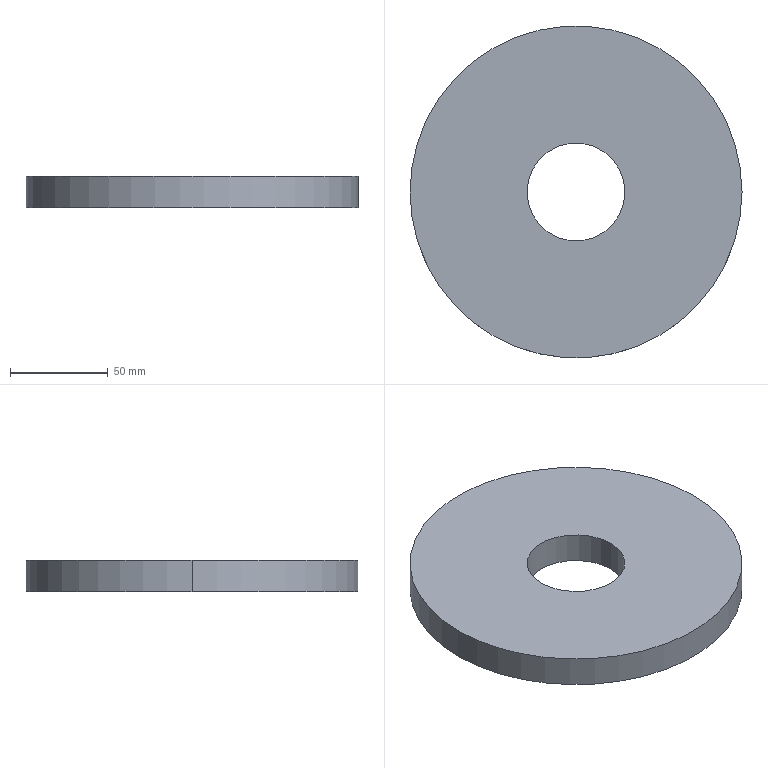Part | SolidWorks | features Extrusion 1 | 1 solid | 6 faces | box 169.5 x 169.5 x 16 mm | volume 329619 mm3 | cylinder 4 | plane 2 | commonest cylinder face diameters 50 x2 169.5 x2
STEP:
#1=CARTESIAN_POINT('',(-25.,0.,16.));
#2=VERTEX_POINT('',#1);
#3=CARTESIAN_POINT('',(25.,0.,16.));
#4=VERTEX_POINT('',#3);
#5=CARTESIAN_POINT('',(0.,0.,16.));
#6=DIRECTION('',(0.,0.,1.));
#7=DIRECTION('',(1.,0.,0.));
#8=AXIS2_PLACEMENT_3D('',#5,#6,#7);
#9=CIRCLE('',#8,25.);
#10=EDGE_CURVE('',#2,#4,#9,.T.);
#11=ORIENTED_EDGE('',*,*,#10,.T.);
#12=CARTESIAN_POINT('',(25.,0.,0.));
#13=VERTEX_POINT('',#12);
#14=CARTESIAN_POINT('',(25.,0.,16.));
#15=DIRECTION('',(0.,0.,-1.));
#16=VECTOR('',#15,1000.);
#17=LINE('',#14,#16);
#18=EDGE_CURVE('',#4,#13,#17,.T.);
#19=ORIENTED_EDGE('',*,*,#18,.T.);
#20=CARTESIAN_POINT('',(-25.,0.,0.));
#21=VERTEX_POINT('',#20);
#22=CARTESIAN_POINT('',(0.,0.,0.));
#23=DIRECTION('',(0.,0.,1.));
#24=DIRECTION('',(1.,0.,0.));
#25=AXIS2_PLACEMENT_3D('',#22,#23,#24);
#26=CIRCLE('',#25,25.);
#27=EDGE_CURVE('',#21,#13,#26,.T.);
#28=ORIENTED_EDGE('',*,*,#27,.F.);
#29=CARTESIAN_POINT('',(-25.,0.,16.));
#30=DIRECTION('',(0.,0.,-1.));
#31=VECTOR('',#30,1000.);
#32=LINE('',#29,#31);
#33=EDGE_CURVE('',#2,#21,#32,.T.);
#34=ORIENTED_EDGE('',*,*,#33,.F.);
#35=EDGE_LOOP('',(#11,#19,#28,#34));
#36=FACE_OUTER_BOUND('',#35,.T.);
#37=CARTESIAN_POINT('',(0.,0.,16.));
#38=DIRECTION('',(0.,0.,-1.));
#39=DIRECTION('',(-1.,0.,0.));
#40=AXIS2_PLACEMENT_3D('',#37,#38,#39);
#41=CYLINDRICAL_SURFACE('',#40,25.);
#42=ADVANCED_FACE('',(#36),#41,.F.);
#43=CARTESIAN_POINT('',(84.75,0.,16.));
#44=VERTEX_POINT('',#43);
#45=CARTESIAN_POINT('',(-84.75,0.,16.));
#46=VERTEX_POINT('',#45);
#47=CARTESIAN_POINT('',(0.,0.,16.));
#48=DIRECTION('',(0.,0.,1.));
#49=DIRECTION('',(1.,0.,0.));
#50=AXIS2_PLACEMENT_3D('',#47,#48,#49);
#51=CIRCLE('',#50,84.75);
#52=EDGE_CURVE('',#44,#46,#51,.T.);
#53=ORIENTED_EDGE('',*,*,#52,.F.);
#54=CARTESIAN_POINT('',(84.75,0.,0.));
#55=VERTEX_POINT('',#54);
#56=CARTESIAN_POINT('',(84.75,0.,16.));
#57=DIRECTION('',(0.,0.,-1.));
#58=VECTOR('',#57,1000.);
#59=LINE('',#56,#58);
#60=EDGE_CURVE('',#44,#55,#59,.T.);
#61=ORIENTED_EDGE('',*,*,#60,.T.);
#62=CARTESIAN_POINT('',(-84.75,0.,0.));
#63=VERTEX_POINT('',#62);
#64=CARTESIAN_POINT('',(0.,0.,0.));
#65=DIRECTION('',(0.,0.,1.));
#66=DIRECTION('',(1.,0.,0.));
#67=AXIS2_PLACEMENT_3D('',#64,#65,#66);
#68=CIRCLE('',#67,84.75);
#69=EDGE_CURVE('',#55,#63,#68,.T.);
#70=ORIENTED_EDGE('',*,*,#69,.T.);
#71=CARTESIAN_POINT('',(-84.75,0.,16.));
#72=DIRECTION('',(0.,0.,-1.));
#73=VECTOR('',#72,1000.);
#74=LINE('',#71,#73);
#75=EDGE_CURVE('',#46,#63,#74,.T.);
#76=ORIENTED_EDGE('',*,*,#75,.F.);
#77=EDGE_LOOP('',(#53,#61,#70,#76));
#78=FACE_OUTER_BOUND('',#77,.T.);
#79=CARTESIAN_POINT('',(0.,0.,16.));
#80=DIRECTION('',(0.,0.,-1.));
#81=DIRECTION('',(-1.,0.,0.));
#82=AXIS2_PLACEMENT_3D('',#79,#80,#81);
#83=CYLINDRICAL_SURFACE('',#82,84.75);
#84=ADVANCED_FACE('',(#78),#83,.T.);
#85=CARTESIAN_POINT('',(0.,0.,16.));
#86=DIRECTION('',(0.,0.,1.));
#87=DIRECTION('',(1.,0.,0.));
#88=AXIS2_PLACEMENT_3D('',#85,#86,#87);
#89=CIRCLE('',#88,84.75);
#90=EDGE_CURVE('',#46,#44,#89,.T.);
#91=ORIENTED_EDGE('',*,*,#90,.T.);
#92=ORIENTED_EDGE('',*,*,#52,.T.);
#93=EDGE_LOOP('',(#91,#92));
#94=FACE_OUTER_BOUND('',#93,.T.);
#95=ORIENTED_EDGE('',*,*,#10,.F.);
#96=CARTESIAN_POINT('',(0.,0.,16.));
#97=DIRECTION('',(0.,0.,1.));
#98=DIRECTION('',(1.,0.,0.));
#99=AXIS2_PLACEMENT_3D('',#96,#97,#98);
#100=CIRCLE('',#99,25.);
#101=EDGE_CURVE('',#4,#2,#100,.T.);
#102=ORIENTED_EDGE('',*,*,#101,.F.);
#103=EDGE_LOOP('',(#95,#102));
#104=FACE_BOUND('',#103,.T.);
#105=CARTESIAN_POINT('',(0.,0.,16.));
#106=DIRECTION('',(0.,0.,1.));
#107=DIRECTION('',(1.,0.,0.));
#108=AXIS2_PLACEMENT_3D('',#105,#106,#107);
#109=PLANE('',#108);
#110=ADVANCED_FACE('',(#94,#104),#109,.T.);
#111=CARTESIAN_POINT('',(0.,0.,0.));
#112=DIRECTION('',(0.,0.,1.));
#113=DIRECTION('',(1.,0.,0.));
#114=AXIS2_PLACEMENT_3D('',#111,#112,#113);
#115=CIRCLE('',#114,84.75);
#116=EDGE_CURVE('',#63,#55,#115,.T.);
#117=ORIENTED_EDGE('',*,*,#116,.F.);
#118=ORIENTED_EDGE('',*,*,#69,.F.);
#119=EDGE_LOOP('',(#117,#118));
#120=FACE_OUTER_BOUND('',#119,.T.);
#121=ORIENTED_EDGE('',*,*,#27,.T.);
#122=CARTESIAN_POINT('',(0.,0.,0.));
#123=DIRECTION('',(0.,0.,1.));
#124=DIRECTION('',(1.,0.,0.));
#125=AXIS2_PLACEMENT_3D('',#122,#123,#124);
#126=CIRCLE('',#125,25.);
#127=EDGE_CURVE('',#13,#21,#126,.T.);
#128=ORIENTED_EDGE('',*,*,#127,.T.);
#129=EDGE_LOOP('',(#121,#128));
#130=FACE_BOUND('',#129,.T.);
#131=CARTESIAN_POINT('',(0.,0.,0.));
#132=DIRECTION('',(0.,0.,1.));
#133=DIRECTION('',(1.,0.,0.));
#134=AXIS2_PLACEMENT_3D('',#131,#132,#133);
#135=PLANE('',#134);
#136=ADVANCED_FACE('',(#120,#130),#135,.F.);
#137=ORIENTED_EDGE('',*,*,#60,.F.);
#138=ORIENTED_EDGE('',*,*,#90,.F.);
#139=ORIENTED_EDGE('',*,*,#75,.T.);
#140=ORIENTED_EDGE('',*,*,#116,.T.);
#141=EDGE_LOOP('',(#137,#138,#139,#140));
#142=FACE_OUTER_BOUND('',#141,.T.);
#143=CARTESIAN_POINT('',(0.,0.,16.));
#144=DIRECTION('',(0.,0.,-1.));
#145=DIRECTION('',(-1.,0.,0.));
#146=AXIS2_PLACEMENT_3D('',#143,#144,#145);
#147=CYLINDRICAL_SURFACE('',#146,84.75);
#148=ADVANCED_FACE('',(#142),#147,.T.);
#149=ORIENTED_EDGE('',*,*,#18,.F.);
#150=ORIENTED_EDGE('',*,*,#101,.T.);
#151=ORIENTED_EDGE('',*,*,#33,.T.);
#152=ORIENTED_EDGE('',*,*,#127,.F.);
#153=EDGE_LOOP('',(#149,#150,#151,#152));
#154=FACE_OUTER_BOUND('',#153,.T.);
#155=CARTESIAN_POINT('',(0.,0.,16.));
#156=DIRECTION('',(0.,0.,-1.));
#157=DIRECTION('',(-1.,0.,0.));
#158=AXIS2_PLACEMENT_3D('',#155,#156,#157);
#159=CYLINDRICAL_SURFACE('',#158,25.);
#160=ADVANCED_FACE('',(#154),#159,.F.);
#161=CLOSED_SHELL('',(#42,#84,#110,#136,#148,#160));
#162=MANIFOLD_SOLID_BREP('',#161);
#163=CARTESIAN_POINT('',(0.,0.,0.));
#164=DIRECTION('',(0.,0.,1.));
#165=DIRECTION('',(1.,0.,0.));
#166=AXIS2_PLACEMENT_3D('',#163,#164,#165);
#167=(LENGTH_UNIT()NAMED_UNIT(*)SI_UNIT(.MILLI.,.METRE.));
#168=UNCERTAINTY_MEASURE_WITH_UNIT(LENGTH_MEASURE(0.00001),#167,'','');
#169=(NAMED_UNIT(*)PLANE_ANGLE_UNIT()SI_UNIT($,.RADIAN.));
#170=(NAMED_UNIT(*)SI_UNIT($,.STERADIAN.)SOLID_ANGLE_UNIT());
#171=(GEOMETRIC_REPRESENTATION_CONTEXT(3)GLOBAL_UNCERTAINTY_ASSIGNED_CONTEXT((#168))GLOBAL_UNIT_ASSIGNED_CONTEXT((#167,#169,#170))REPRESENTATION_CONTEXT('',''));
#172=ADVANCED_BREP_SHAPE_REPRESENTATION('',(#162,#166),#171);